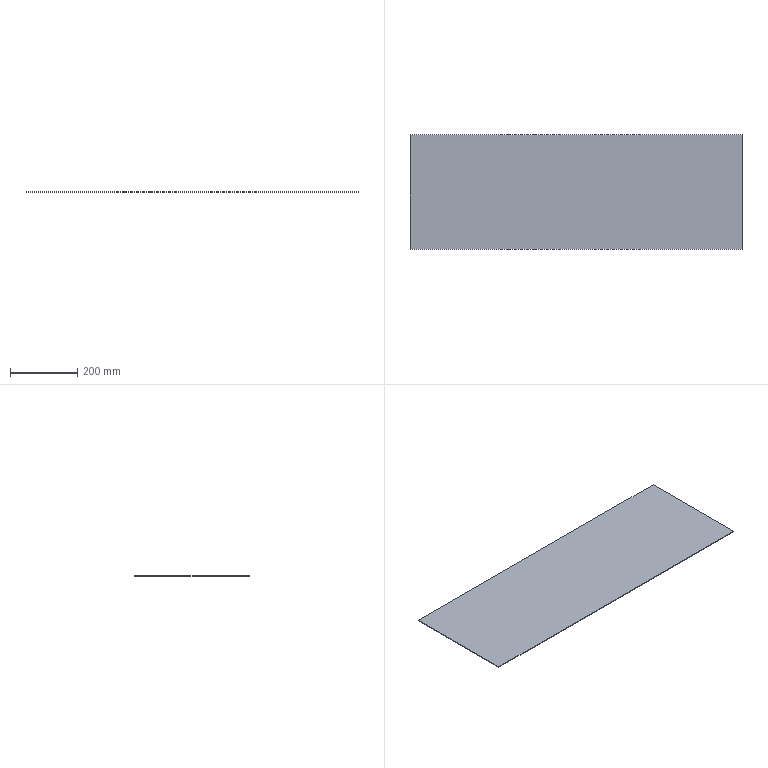Part | SolidWorks | features Extrusion 1 | 1 solid | 6 faces | box 990 x 340 x 2 mm | volume 673200 mm3 | plane 6
STEP:
#1=CARTESIAN_POINT('',(-286.503,182.483,0.));
#2=VERTEX_POINT('',#1);
#3=CARTESIAN_POINT('',(-286.503,-157.517,0.));
#4=VERTEX_POINT('',#3);
#5=CARTESIAN_POINT('',(-286.503,182.483,0.));
#6=DIRECTION('',(0.,-1.,0.));
#7=VECTOR('',#6,1000.);
#8=LINE('',#5,#7);
#9=EDGE_CURVE('',#2,#4,#8,.T.);
#10=ORIENTED_EDGE('',*,*,#9,.T.);
#11=CARTESIAN_POINT('',(-286.503,-157.517,2.));
#12=VERTEX_POINT('',#11);
#13=CARTESIAN_POINT('',(-286.503,-157.517,2.));
#14=DIRECTION('',(0.,0.,-1.));
#15=VECTOR('',#14,1000.);
#16=LINE('',#13,#15);
#17=EDGE_CURVE('',#12,#4,#16,.T.);
#18=ORIENTED_EDGE('',*,*,#17,.F.);
#19=CARTESIAN_POINT('',(-286.503,182.483,2.));
#20=VERTEX_POINT('',#19);
#21=CARTESIAN_POINT('',(-286.503,182.483,2.));
#22=DIRECTION('',(0.,-1.,0.));
#23=VECTOR('',#22,1000.);
#24=LINE('',#21,#23);
#25=EDGE_CURVE('',#20,#12,#24,.T.);
#26=ORIENTED_EDGE('',*,*,#25,.F.);
#27=CARTESIAN_POINT('',(-286.503,182.483,2.));
#28=DIRECTION('',(0.,0.,-1.));
#29=VECTOR('',#28,1000.);
#30=LINE('',#27,#29);
#31=EDGE_CURVE('',#20,#2,#30,.T.);
#32=ORIENTED_EDGE('',*,*,#31,.T.);
#33=EDGE_LOOP('',(#10,#18,#26,#32));
#34=FACE_OUTER_BOUND('',#33,.T.);
#35=CARTESIAN_POINT('',(-286.503,182.483,2.));
#36=DIRECTION('',(1.,0.,0.));
#37=DIRECTION('',(0.,0.,-1.));
#38=AXIS2_PLACEMENT_3D('',#35,#36,#37);
#39=PLANE('',#38);
#40=ADVANCED_FACE('',(#34),#39,.F.);
#41=CARTESIAN_POINT('',(703.497,-157.517,0.));
#42=VERTEX_POINT('',#41);
#43=CARTESIAN_POINT('',(-286.503,-157.517,0.));
#44=DIRECTION('',(1.,0.,0.));
#45=VECTOR('',#44,1000.);
#46=LINE('',#43,#45);
#47=EDGE_CURVE('',#4,#42,#46,.T.);
#48=ORIENTED_EDGE('',*,*,#47,.T.);
#49=CARTESIAN_POINT('',(703.497,-157.517,2.));
#50=VERTEX_POINT('',#49);
#51=CARTESIAN_POINT('',(703.497,-157.517,2.));
#52=DIRECTION('',(0.,0.,-1.));
#53=VECTOR('',#52,1000.);
#54=LINE('',#51,#53);
#55=EDGE_CURVE('',#50,#42,#54,.T.);
#56=ORIENTED_EDGE('',*,*,#55,.F.);
#57=CARTESIAN_POINT('',(-286.503,-157.517,2.));
#58=DIRECTION('',(1.,0.,0.));
#59=VECTOR('',#58,1000.);
#60=LINE('',#57,#59);
#61=EDGE_CURVE('',#12,#50,#60,.T.);
#62=ORIENTED_EDGE('',*,*,#61,.F.);
#63=ORIENTED_EDGE('',*,*,#17,.T.);
#64=EDGE_LOOP('',(#48,#56,#62,#63));
#65=FACE_OUTER_BOUND('',#64,.T.);
#66=CARTESIAN_POINT('',(-286.503,-157.517,2.));
#67=DIRECTION('',(0.,1.,0.));
#68=DIRECTION('',(-1.,0.,0.));
#69=AXIS2_PLACEMENT_3D('',#66,#67,#68);
#70=PLANE('',#69);
#71=ADVANCED_FACE('',(#65),#70,.F.);
#72=CARTESIAN_POINT('',(703.497,182.483,0.));
#73=VERTEX_POINT('',#72);
#74=CARTESIAN_POINT('',(703.497,182.483,0.));
#75=DIRECTION('',(0.,1.,0.));
#76=VECTOR('',#75,1000.);
#77=LINE('',#74,#76);
#78=EDGE_CURVE('',#42,#73,#77,.T.);
#79=ORIENTED_EDGE('',*,*,#78,.T.);
#80=CARTESIAN_POINT('',(703.497,182.483,2.));
#81=VERTEX_POINT('',#80);
#82=CARTESIAN_POINT('',(703.497,182.483,2.));
#83=DIRECTION('',(0.,0.,-1.));
#84=VECTOR('',#83,1000.);
#85=LINE('',#82,#84);
#86=EDGE_CURVE('',#81,#73,#85,.T.);
#87=ORIENTED_EDGE('',*,*,#86,.F.);
#88=CARTESIAN_POINT('',(703.497,182.483,2.));
#89=DIRECTION('',(0.,1.,0.));
#90=VECTOR('',#89,1000.);
#91=LINE('',#88,#90);
#92=EDGE_CURVE('',#50,#81,#91,.T.);
#93=ORIENTED_EDGE('',*,*,#92,.F.);
#94=ORIENTED_EDGE('',*,*,#55,.T.);
#95=EDGE_LOOP('',(#79,#87,#93,#94));
#96=FACE_OUTER_BOUND('',#95,.T.);
#97=CARTESIAN_POINT('',(703.497,182.483,2.));
#98=DIRECTION('',(-1.,0.,0.));
#99=DIRECTION('',(0.,0.,1.));
#100=AXIS2_PLACEMENT_3D('',#97,#98,#99);
#101=PLANE('',#100);
#102=ADVANCED_FACE('',(#96),#101,.F.);
#103=CARTESIAN_POINT('',(-286.503,182.483,0.));
#104=DIRECTION('',(-1.,0.,0.));
#105=VECTOR('',#104,1000.);
#106=LINE('',#103,#105);
#107=EDGE_CURVE('',#73,#2,#106,.T.);
#108=ORIENTED_EDGE('',*,*,#107,.T.);
#109=ORIENTED_EDGE('',*,*,#31,.F.);
#110=CARTESIAN_POINT('',(-286.503,182.483,2.));
#111=DIRECTION('',(-1.,0.,0.));
#112=VECTOR('',#111,1000.);
#113=LINE('',#110,#112);
#114=EDGE_CURVE('',#81,#20,#113,.T.);
#115=ORIENTED_EDGE('',*,*,#114,.F.);
#116=ORIENTED_EDGE('',*,*,#86,.T.);
#117=EDGE_LOOP('',(#108,#109,#115,#116));
#118=FACE_OUTER_BOUND('',#117,.T.);
#119=CARTESIAN_POINT('',(-286.503,182.483,2.));
#120=DIRECTION('',(0.,-1.,0.));
#121=DIRECTION('',(0.,0.,-1.));
#122=AXIS2_PLACEMENT_3D('',#119,#120,#121);
#123=PLANE('',#122);
#124=ADVANCED_FACE('',(#118),#123,.F.);
#125=ORIENTED_EDGE('',*,*,#25,.T.);
#126=ORIENTED_EDGE('',*,*,#61,.T.);
#127=ORIENTED_EDGE('',*,*,#92,.T.);
#128=ORIENTED_EDGE('',*,*,#114,.T.);
#129=EDGE_LOOP('',(#125,#126,#127,#128));
#130=FACE_OUTER_BOUND('',#129,.T.);
#131=CARTESIAN_POINT('',(0.,0.,2.));
#132=DIRECTION('',(0.,0.,1.));
#133=DIRECTION('',(1.,0.,0.));
#134=AXIS2_PLACEMENT_3D('',#131,#132,#133);
#135=PLANE('',#134);
#136=ADVANCED_FACE('',(#130),#135,.T.);
#137=ORIENTED_EDGE('',*,*,#9,.F.);
#138=ORIENTED_EDGE('',*,*,#107,.F.);
#139=ORIENTED_EDGE('',*,*,#78,.F.);
#140=ORIENTED_EDGE('',*,*,#47,.F.);
#141=EDGE_LOOP('',(#137,#138,#139,#140));
#142=FACE_OUTER_BOUND('',#141,.T.);
#143=CARTESIAN_POINT('',(0.,0.,0.));
#144=DIRECTION('',(0.,0.,1.));
#145=DIRECTION('',(1.,0.,0.));
#146=AXIS2_PLACEMENT_3D('',#143,#144,#145);
#147=PLANE('',#146);
#148=ADVANCED_FACE('',(#142),#147,.F.);
#149=CLOSED_SHELL('',(#40,#71,#102,#124,#136,#148));
#150=MANIFOLD_SOLID_BREP('',#149);
#151=CARTESIAN_POINT('',(0.,0.,0.));
#152=DIRECTION('',(0.,0.,1.));
#153=DIRECTION('',(1.,0.,0.));
#154=AXIS2_PLACEMENT_3D('',#151,#152,#153);
#155=(LENGTH_UNIT()NAMED_UNIT(*)SI_UNIT(.MILLI.,.METRE.));
#156=UNCERTAINTY_MEASURE_WITH_UNIT(LENGTH_MEASURE(0.00001),#155,'','');
#157=(NAMED_UNIT(*)PLANE_ANGLE_UNIT()SI_UNIT($,.RADIAN.));
#158=(NAMED_UNIT(*)SI_UNIT($,.STERADIAN.)SOLID_ANGLE_UNIT());
#159=(GEOMETRIC_REPRESENTATION_CONTEXT(3)GLOBAL_UNCERTAINTY_ASSIGNED_CONTEXT((#156))GLOBAL_UNIT_ASSIGNED_CONTEXT((#155,#157,#158))REPRESENTATION_CONTEXT('',''));
#160=ADVANCED_BREP_SHAPE_REPRESENTATION('',(#150,#154),#159);